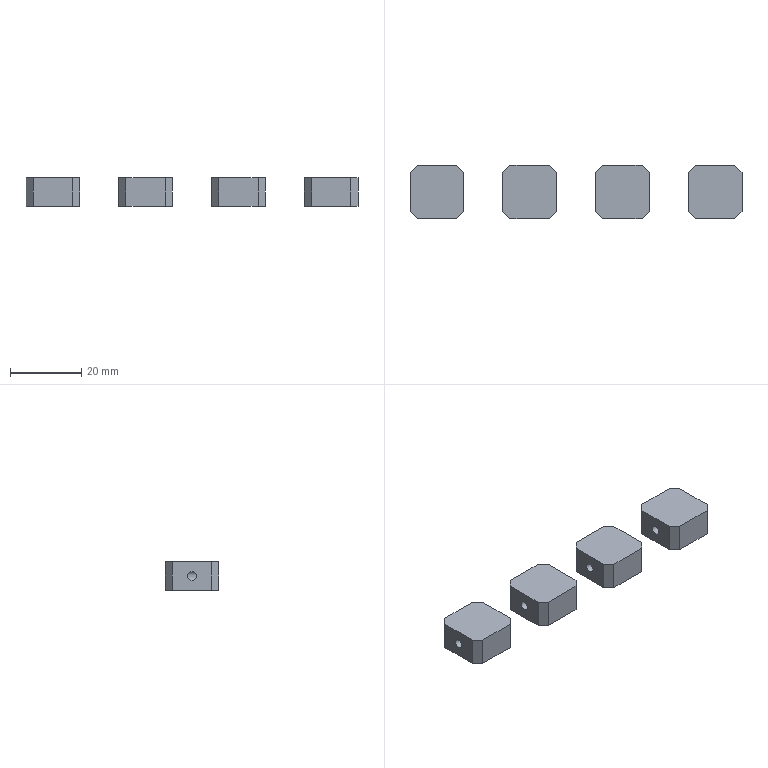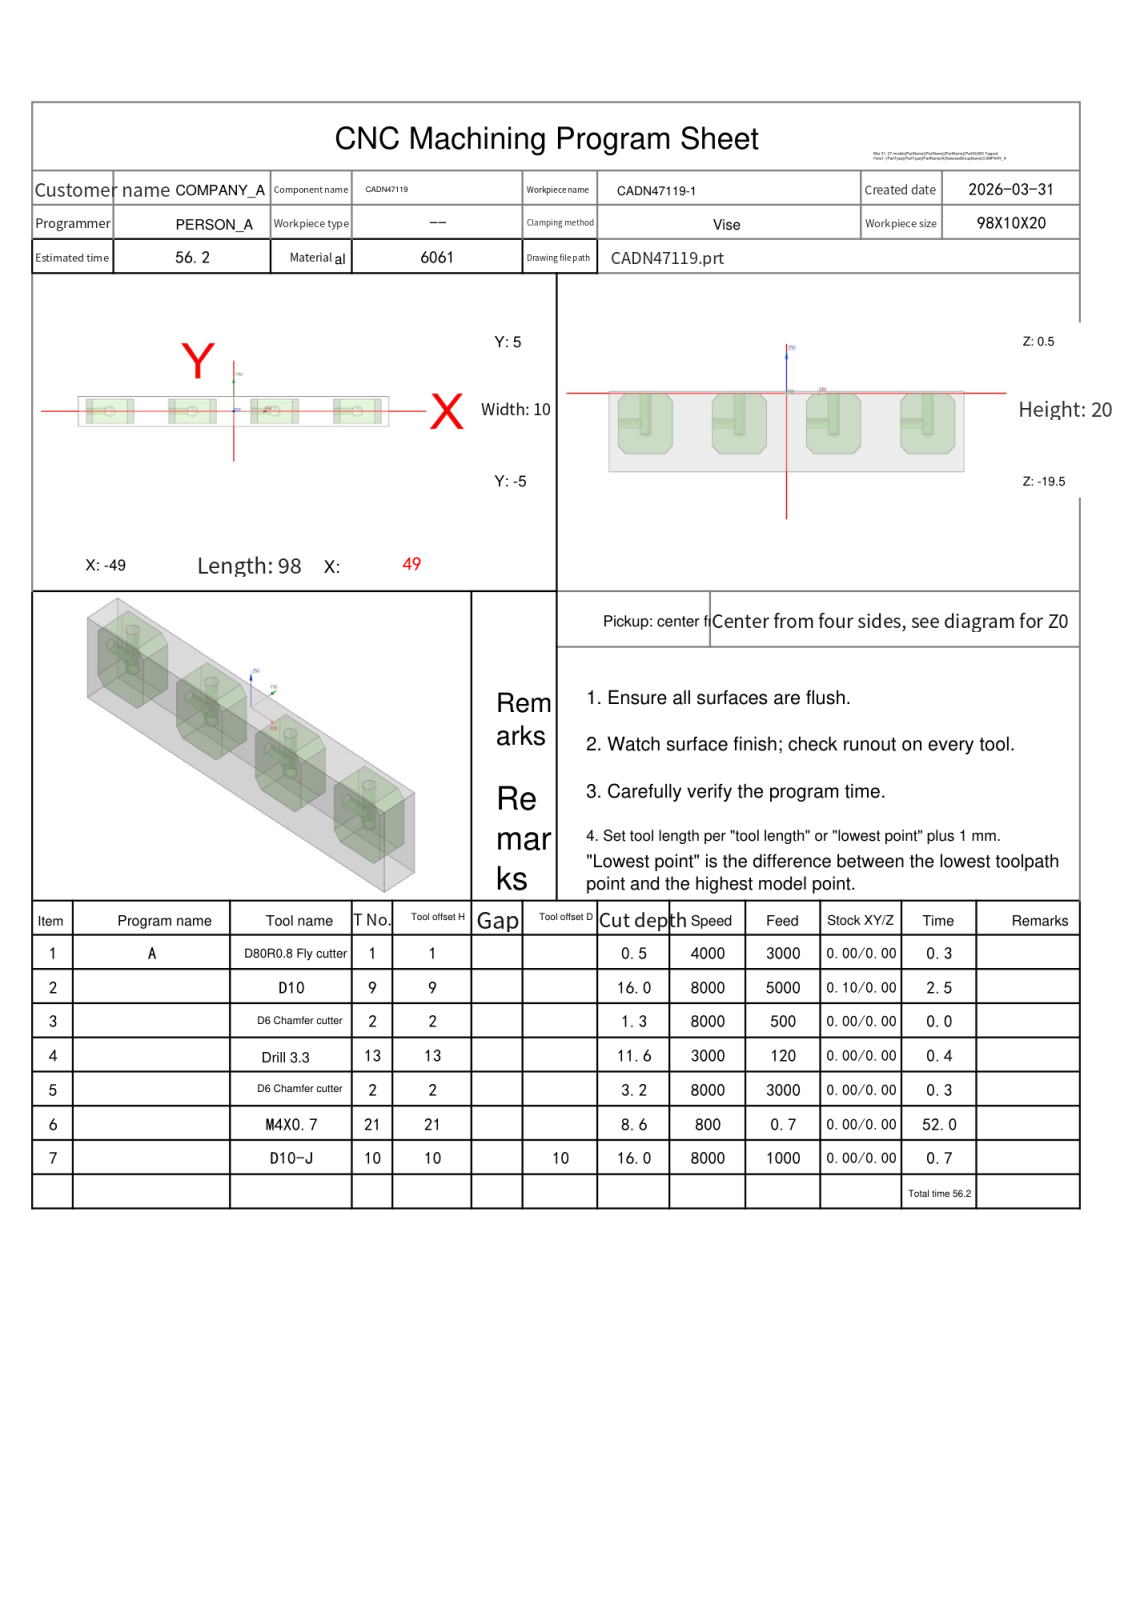NC program | NX | posted by the shop | part box 93 x 15 x 8 mm
Whole program, first 1516 of 2116 lines:
%
O0001
(Machine time: 103.83 MIN)
(===Total Tool:6===)
(T1=D80R0.8 Fly cutter D=80.  R=0.8  D-  H01 Z=-0.   )
(T9=D10     D=10.  R=0.   D-  H09 Z=-15.5 )
(T2=D6 Chamfer cutter   D=6.   R=0.   D-  H02 Z=-2.7  )
(T13=Drill 3.3  D=3.3  DR_a=118 D-  H13 Z=-11.09)
(T21=M4X0.7 D=3.3  DR_a=180 D-  H21 Z=-8.1  )
(T10=D10-J  D=10.  R=0.   D10 H10 Z=-15.5 )
G80 G90 G17 G49 G40
G91 G28 Z0
M01
N1 T01 M06
(D80R0.8 Fly cutter  D=80. R=0.8 H=01 ce=0.20 di=0.10)
G00 G90 G54 X91.5 Y0.0 M03 S4000
G43 H01 Z20.
M08
Z2.1
G01 Z.1 F3000.
X86.5
X-86.5
X-91.5
Z2.1
G00 Z20.
G00 G90 X91.5 Y0.0 M03 S4000
Z20.
Z2.
G01 Z0.0 F1000.
X86.5
X-86.5
X-91.5
Z2.
G00 Z20.
G91 G28 Z0.0
M05
M09
G91 G28 Z0.0
M01
N2 T09 M06
(D10  D=10. R=0. H=09 ce=0.10 di=0.00)
G00 G90 G54 X13. Y9.1 M03 S8000
G43 H09 Z20.
M08
Z.5
G01 X20.5 Z.452 F5000.
G02 X25.6 Y4. Z.401 I0.0 J-5.1
G01 Y-4. Z.349
G02 X20.5 Y-9.1 Z.298 I-5.1 J0.0
G01 X5.5 Z.202
G02 X.4 Y-4. Z.151 I0.0 J5.1
G01 Y4. Z.099
G02 X5.5 Y9.1 Z.048 I5.1 J0.0
G01 X20.5 Z-.048
G02 X25.6 Y4. Z-.099 I0.0 J-5.1
G01 Y-4. Z-.151
G02 X20.5 Y-9.1 Z-.202 I-5.1 J0.0
G01 X5.5 Z-.298
G02 X.4 Y-4. Z-.349 I0.0 J5.1
G01 Y4. Z-.401
G02 X5.5 Y9.1 Z-.452 I5.1 J0.0
G01 X20.5 Z-.548
G02 X25.6 Y4. Z-.599 I0.0 J-5.1
G01 Y-4. Z-.651
G02 X20.5 Y-9.1 Z-.702 I-5.1 J0.0
G01 X5.5 Z-.798
G02 X.4 Y-4. Z-.849 I0.0 J5.1
G01 Y4. Z-.901
G02 X5.5 Y9.1 Z-.952 I5.1 J0.0
G01 X20.5 Z-1.048
G02 X25.6 Y4. Z-1.099 I0.0 J-5.1
G01 Y-4. Z-1.151
G02 X20.5 Y-9.1 Z-1.202 I-5.1 J0.0
G01 X5.5 Z-1.298
G02 X.4 Y-4. Z-1.349 I0.0 J5.1
G01 Y4. Z-1.401
G02 X5.5 Y9.1 Z-1.452 I5.1 J0.0
G01 X20.5 Z-1.548
G02 X25.6 Y4. Z-1.599 I0.0 J-5.1
G01 Y-4. Z-1.651
G02 X20.5 Y-9.1 Z-1.702 I-5.1 J0.0
G01 X5.5 Z-1.798
G02 X.4 Y-4. Z-1.849 I0.0 J5.1
G01 Y4. Z-1.901
G02 X5.5 Y9.1 Z-1.952 I5.1 J0.0
G01 X20.5 Z-2.048
G02 X25.6 Y4. Z-2.099 I0.0 J-5.1
G01 Y-4. Z-2.151
G02 X20.5 Y-9.1 Z-2.202 I-5.1 J0.0
G01 X5.5 Z-2.298
G02 X.4 Y-4. Z-2.349 I0.0 J5.1
G01 Y4. Z-2.401
G02 X5.5 Y9.1 Z-2.452 I5.1 J0.0
G01 X20.5 Z-2.548
G02 X25.6 Y4. Z-2.599 I0.0 J-5.1
G01 Y-4. Z-2.651
G02 X20.5 Y-9.1 Z-2.702 I-5.1 J0.0
G01 X5.5 Z-2.798
G02 X.4 Y-4. Z-2.849 I0.0 J5.1
G01 Y4. Z-2.901
G02 X5.5 Y9.1 Z-2.952 I5.1 J0.0
G01 X20.5 Z-3.048
G02 X25.6 Y4. Z-3.099 I0.0 J-5.1
G01 Y-4. Z-3.151
G02 X20.5 Y-9.1 Z-3.202 I-5.1 J0.0
G01 X5.5 Z-3.298
G02 X.4 Y-4. Z-3.349 I0.0 J5.1
G01 Y4. Z-3.401
G02 X5.5 Y9.1 Z-3.452 I5.1 J0.0
G01 X20.5 Z-3.548
G02 X25.6 Y4. Z-3.599 I0.0 J-5.1
G01 Y-4. Z-3.651
G02 X20.5 Y-9.1 Z-3.702 I-5.1 J0.0
G01 X5.5 Z-3.798
G02 X.4 Y-4. Z-3.849 I0.0 J5.1
G01 Y4. Z-3.901
G02 X5.5 Y9.1 Z-3.952 I5.1 J0.0
G01 X20.5 Z-4.048
G02 X25.6 Y4. Z-4.099 I0.0 J-5.1
G01 Y-4. Z-4.151
G02 X20.5 Y-9.1 Z-4.202 I-5.1 J0.0
G01 X5.5 Z-4.298
G02 X.4 Y-4. Z-4.349 I0.0 J5.1
G01 Y4. Z-4.401
G02 X5.5 Y9.1 Z-4.452 I5.1 J0.0
G01 X20.5 Z-4.548
G02 X25.6 Y4. Z-4.599 I0.0 J-5.1
G01 Y-4. Z-4.651
G02 X20.5 Y-9.1 Z-4.702 I-5.1 J0.0
G01 X5.5 Z-4.798
G02 X.4 Y-4. Z-4.849 I0.0 J5.1
G01 Y4. Z-4.901
G02 X5.5 Y9.1 Z-4.952 I5.1 J0.0
G01 X20.5 Z-5.048
G02 X25.6 Y4. Z-5.099 I0.0 J-5.1
G01 Y-4. Z-5.151
G02 X20.5 Y-9.1 Z-5.202 I-5.1 J0.0
G01 X5.5 Z-5.298
G02 X.4 Y-4. Z-5.349 I0.0 J5.1
G01 Y4. Z-5.401
G02 X5.5 Y9.1 Z-5.452 I5.1 J0.0
G01 X20.5 Z-5.548
G02 X25.6 Y4. Z-5.599 I0.0 J-5.1
G01 Y-4. Z-5.651
G02 X20.5 Y-9.1 Z-5.702 I-5.1 J0.0
G01 X5.5 Z-5.798
G02 X.4 Y-4. Z-5.849 I0.0 J5.1
G01 Y4. Z-5.901
G02 X5.5 Y9.1 Z-5.952 I5.1 J0.0
G01 X20.5 Z-6.048
G02 X25.6 Y4. Z-6.099 I0.0 J-5.1
G01 Y-4. Z-6.151
G02 X20.5 Y-9.1 Z-6.202 I-5.1 J0.0
G01 X5.5 Z-6.298
G02 X.4 Y-4. Z-6.349 I0.0 J5.1
G01 Y4. Z-6.401
G02 X5.5 Y9.1 Z-6.452 I5.1 J0.0
G01 X20.5 Z-6.548
G02 X25.6 Y4. Z-6.599 I0.0 J-5.1
G01 Y-4. Z-6.651
G02 X20.5 Y-9.1 Z-6.702 I-5.1 J0.0
G01 X5.5 Z-6.798
G02 X.4 Y-4. Z-6.849 I0.0 J5.1
G01 Y4. Z-6.901
G02 X5.5 Y9.1 Z-6.952 I5.1 J0.0
G01 X20.5 Z-7.048
G02 X25.6 Y4. Z-7.099 I0.0 J-5.1
G01 Y-4. Z-7.151
G02 X20.5 Y-9.1 Z-7.202 I-5.1 J0.0
G01 X5.5 Z-7.298
G02 X.4 Y-4. Z-7.349 I0.0 J5.1
G01 Y4. Z-7.401
G02 X5.5 Y9.1 Z-7.452 I5.1 J0.0
G01 X20.5 Z-7.548
G02 X25.6 Y4. Z-7.599 I0.0 J-5.1
G01 Y-4. Z-7.651
G02 X20.5 Y-9.1 Z-7.702 I-5.1 J0.0
G01 X5.5 Z-7.798
G02 X.4 Y-4. Z-7.849 I0.0 J5.1
G01 Y4. Z-7.901
G02 X5.5 Y9.1 Z-7.952 I5.1 J0.0
G01 X20.5 Z-8.048
G02 X25.6 Y4. Z-8.099 I0.0 J-5.1
G01 Y-4. Z-8.151
G02 X20.5 Y-9.1 Z-8.202 I-5.1 J0.0
G01 X5.5 Z-8.298
G02 X.4 Y-4. Z-8.349 I0.0 J5.1
G01 Y4. Z-8.401
G02 X5.5 Y9.1 Z-8.452 I5.1 J0.0
G01 X20.5 Z-8.548
G02 X25.6 Y4. Z-8.599 I0.0 J-5.1
G01 Y-4. Z-8.651
G02 X20.5 Y-9.1 Z-8.702 I-5.1 J0.0
G01 X5.5 Z-8.798
G02 X.4 Y-4. Z-8.849 I0.0 J5.1
G01 Y4. Z-8.901
G02 X5.5 Y9.1 Z-8.952 I5.1 J0.0
G01 X20.5 Z-9.048
G02 X25.6 Y4. Z-9.099 I0.0 J-5.1
G01 Y-4. Z-9.151
G02 X20.5 Y-9.1 Z-9.202 I-5.1 J0.0
G01 X5.5 Z-9.298
G02 X.4 Y-4. Z-9.349 I0.0 J5.1
G01 Y4. Z-9.401
G02 X5.5 Y9.1 Z-9.452 I5.1 J0.0
G01 X20.5 Z-9.548
G02 X25.6 Y4. Z-9.599 I0.0 J-5.1
G01 Y-4. Z-9.651
G02 X20.5 Y-9.1 Z-9.702 I-5.1 J0.0
G01 X5.5 Z-9.798
G02 X.4 Y-4. Z-9.849 I0.0 J5.1
G01 Y4. Z-9.901
G02 X5.5 Y9.1 Z-9.952 I5.1 J0.0
G01 X20.5 Z-10.048
G02 X25.6 Y4. Z-10.099 I0.0 J-5.1
G01 Y-4. Z-10.151
G02 X20.5 Y-9.1 Z-10.202 I-5.1 J0.0
G01 X5.5 Z-10.298
G02 X.4 Y-4. Z-10.349 I0.0 J5.1
G01 Y4. Z-10.401
G02 X5.5 Y9.1 Z-10.452 I5.1 J0.0
G01 X20.5 Z-10.548
G02 X25.6 Y4. Z-10.599 I0.0 J-5.1
G01 Y-4. Z-10.651
G02 X20.5 Y-9.1 Z-10.702 I-5.1 J0.0
G01 X5.5 Z-10.798
G02 X.4 Y-4. Z-10.849 I0.0 J5.1
G01 Y4. Z-10.901
G02 X5.5 Y9.1 Z-10.952 I5.1 J0.0
G01 X20.5 Z-11.048
G02 X25.6 Y4. Z-11.099 I0.0 J-5.1
G01 Y-4. Z-11.151
G02 X20.5 Y-9.1 Z-11.202 I-5.1 J0.0
G01 X5.5 Z-11.298
G02 X.4 Y-4. Z-11.349 I0.0 J5.1
G01 Y4. Z-11.401
G02 X5.5 Y9.1 Z-11.452 I5.1 J0.0
G01 X20.5 Z-11.548
G02 X25.6 Y4. Z-11.599 I0.0 J-5.1
G01 Y-4. Z-11.651
G02 X20.5 Y-9.1 Z-11.702 I-5.1 J0.0
G01 X5.5 Z-11.798
G02 X.4 Y-4. Z-11.849 I0.0 J5.1
G01 Y4. Z-11.901
G02 X5.5 Y9.1 Z-11.952 I5.1 J0.0
G01 X20.5 Z-12.048
G02 X25.6 Y4. Z-12.099 I0.0 J-5.1
G01 Y-4. Z-12.151
G02 X20.5 Y-9.1 Z-12.202 I-5.1 J0.0
G01 X5.5 Z-12.298
G02 X.4 Y-4. Z-12.349 I0.0 J5.1
G01 Y4. Z-12.401
G02 X5.5 Y9.1 Z-12.452 I5.1 J0.0
G01 X20.5 Z-12.548
G02 X25.6 Y4. Z-12.599 I0.0 J-5.1
G01 Y-4. Z-12.651
G02 X20.5 Y-9.1 Z-12.702 I-5.1 J0.0
G01 X5.5 Z-12.798
G02 X.4 Y-4. Z-12.849 I0.0 J5.1
G01 Y4. Z-12.901
G02 X5.5 Y9.1 Z-12.952 I5.1 J0.0
G01 X20.5 Z-13.048
G02 X25.6 Y4. Z-13.099 I0.0 J-5.1
G01 Y-4. Z-13.151
G02 X20.5 Y-9.1 Z-13.202 I-5.1 J0.0
G01 X5.5 Z-13.298
G02 X.4 Y-4. Z-13.349 I0.0 J5.1
G01 Y4. Z-13.401
G02 X5.5 Y9.1 Z-13.452 I5.1 J0.0
G01 X20.5 Z-13.548
G02 X25.6 Y4. Z-13.599 I0.0 J-5.1
G01 Y-4. Z-13.651
G02 X20.5 Y-9.1 Z-13.702 I-5.1 J0.0
G01 X5.5 Z-13.798
G02 X.4 Y-4. Z-13.849 I0.0 J5.1
G01 Y4. Z-13.901
G02 X5.5 Y9.1 Z-13.952 I5.1 J0.0
G01 X20.5 Z-14.048
G02 X25.6 Y4. Z-14.099 I0.0 J-5.1
G01 Y-4. Z-14.151
G02 X20.5 Y-9.1 Z-14.202 I-5.1 J0.0
G01 X5.5 Z-14.298
G02 X.4 Y-4. Z-14.349 I0.0 J5.1
G01 Y4. Z-14.401
G02 X5.5 Y9.1 Z-14.452 I5.1 J0.0
G01 X20.5 Z-14.548
G02 X25.6 Y4. Z-14.599 I0.0 J-5.1
G01 Y-4. Z-14.651
G02 X20.5 Y-9.1 Z-14.702 I-5.1 J0.0
G01 X5.5 Z-14.798
G02 X.4 Y-4. Z-14.849 I0.0 J5.1
G01 Y4. Z-14.901
G02 X5.5 Y9.1 Z-14.952 I5.1 J0.0
G01 X20.5 Z-15.048
G02 X25.6 Y4. Z-15.099 I0.0 J-5.1
G01 Y-4. Z-15.151
G02 X20.5 Y-9.1 Z-15.202 I-5.1 J0.0
G01 X5.5 Z-15.298
G02 X.4 Y-4. Z-15.349 I0.0 J5.1
G01 Y4. Z-15.401
G02 X5.5 Y9.1 Z-15.452 I5.1 J0.0
G01 X13. Z-15.5
X20.5
G02 X25.6 Y4. I0.0 J-5.1
G01 Y-4.
G02 X20.5 Y-9.1 I-5.1 J0.0
G01 X5.5
G02 X.4 Y-4. I0.0 J5.1
G01 Y4.
G02 X5.5 Y9.1 I5.1 J0.0
G01 X13.
X13.5
Z-14.5
G00 Z20.
X39.
Z.5
G01 X46.5 Z.452
G02 X51.6 Y4. Z.401 I0.0 J-5.1
G01 Y-4. Z.349
G02 X46.5 Y-9.1 Z.298 I-5.1 J0.0
G01 X31.5 Z.202
G02 X26.4 Y-4. Z.151 I0.0 J5.1
G01 Y4. Z.099
G02 X31.5 Y9.1 Z.048 I5.1 J0.0
G01 X46.5 Z-.048
G02 X51.6 Y4. Z-.099 I0.0 J-5.1
G01 Y-4. Z-.151
G02 X46.5 Y-9.1 Z-.202 I-5.1 J0.0
G01 X31.5 Z-.298
G02 X26.4 Y-4. Z-.349 I0.0 J5.1
G01 Y4. Z-.401
G02 X31.5 Y9.1 Z-.452 I5.1 J0.0
G01 X46.5 Z-.548
G02 X51.6 Y4. Z-.599 I0.0 J-5.1
G01 Y-4. Z-.651
G02 X46.5 Y-9.1 Z-.702 I-5.1 J0.0
G01 X31.5 Z-.798
G02 X26.4 Y-4. Z-.849 I0.0 J5.1
G01 Y4. Z-.901
G02 X31.5 Y9.1 Z-.952 I5.1 J0.0
G01 X46.5 Z-1.048
G02 X51.6 Y4. Z-1.099 I0.0 J-5.1
G01 Y-4. Z-1.151
G02 X46.5 Y-9.1 Z-1.202 I-5.1 J0.0
G01 X31.5 Z-1.298
G02 X26.4 Y-4. Z-1.349 I0.0 J5.1
G01 Y4. Z-1.401
G02 X31.5 Y9.1 Z-1.452 I5.1 J0.0
G01 X46.5 Z-1.548
G02 X51.6 Y4. Z-1.599 I0.0 J-5.1
G01 Y-4. Z-1.651
G02 X46.5 Y-9.1 Z-1.702 I-5.1 J0.0
G01 X31.5 Z-1.798
G02 X26.4 Y-4. Z-1.849 I0.0 J5.1
G01 Y4. Z-1.901
G02 X31.5 Y9.1 Z-1.952 I5.1 J0.0
G01 X46.5 Z-2.048
G02 X51.6 Y4. Z-2.099 I0.0 J-5.1
G01 Y-4. Z-2.151
G02 X46.5 Y-9.1 Z-2.202 I-5.1 J0.0
G01 X31.5 Z-2.298
G02 X26.4 Y-4. Z-2.349 I0.0 J5.1
G01 Y4. Z-2.401
G02 X31.5 Y9.1 Z-2.452 I5.1 J0.0
G01 X46.5 Z-2.548
G02 X51.6 Y4. Z-2.599 I0.0 J-5.1
G01 Y-4. Z-2.651
G02 X46.5 Y-9.1 Z-2.702 I-5.1 J0.0
G01 X31.5 Z-2.798
G02 X26.4 Y-4. Z-2.849 I0.0 J5.1
G01 Y4. Z-2.901
G02 X31.5 Y9.1 Z-2.952 I5.1 J0.0
G01 X46.5 Z-3.048
G02 X51.6 Y4. Z-3.099 I0.0 J-5.1
G01 Y-4. Z-3.151
G02 X46.5 Y-9.1 Z-3.202 I-5.1 J0.0
G01 X31.5 Z-3.298
G02 X26.4 Y-4. Z-3.349 I0.0 J5.1
G01 Y4. Z-3.401
G02 X31.5 Y9.1 Z-3.452 I5.1 J0.0
G01 X46.5 Z-3.548
G02 X51.6 Y4. Z-3.599 I0.0 J-5.1
G01 Y-4. Z-3.651
G02 X46.5 Y-9.1 Z-3.702 I-5.1 J0.0
G01 X31.5 Z-3.798
G02 X26.4 Y-4. Z-3.849 I0.0 J5.1
G01 Y4. Z-3.901
G02 X31.5 Y9.1 Z-3.952 I5.1 J0.0
G01 X46.5 Z-4.048
G02 X51.6 Y4. Z-4.099 I0.0 J-5.1
G01 Y-4. Z-4.151
G02 X46.5 Y-9.1 Z-4.202 I-5.1 J0.0
G01 X31.5 Z-4.298
G02 X26.4 Y-4. Z-4.349 I0.0 J5.1
G01 Y4. Z-4.401
G02 X31.5 Y9.1 Z-4.452 I5.1 J0.0
G01 X46.5 Z-4.548
G02 X51.6 Y4. Z-4.599 I0.0 J-5.1
G01 Y-4. Z-4.651
G02 X46.5 Y-9.1 Z-4.702 I-5.1 J0.0
G01 X31.5 Z-4.798
G02 X26.4 Y-4. Z-4.849 I0.0 J5.1
G01 Y4. Z-4.901
G02 X31.5 Y9.1 Z-4.952 I5.1 J0.0
G01 X46.5 Z-5.048
G02 X51.6 Y4. Z-5.099 I0.0 J-5.1
G01 Y-4. Z-5.151
G02 X46.5 Y-9.1 Z-5.202 I-5.1 J0.0
G01 X31.5 Z-5.298
G02 X26.4 Y-4. Z-5.349 I0.0 J5.1
G01 Y4. Z-5.401
G02 X31.5 Y9.1 Z-5.452 I5.1 J0.0
G01 X46.5 Z-5.548
G02 X51.6 Y4. Z-5.599 I0.0 J-5.1
G01 Y-4. Z-5.651
G02 X46.5 Y-9.1 Z-5.702 I-5.1 J0.0
G01 X31.5 Z-5.798
G02 X26.4 Y-4. Z-5.849 I0.0 J5.1
G01 Y4. Z-5.901
G02 X31.5 Y9.1 Z-5.952 I5.1 J0.0
G01 X46.5 Z-6.048
G02 X51.6 Y4. Z-6.099 I0.0 J-5.1
G01 Y-4. Z-6.151
G02 X46.5 Y-9.1 Z-6.202 I-5.1 J0.0
G01 X31.5 Z-6.298
G02 X26.4 Y-4. Z-6.349 I0.0 J5.1
G01 Y4. Z-6.401
G02 X31.5 Y9.1 Z-6.452 I5.1 J0.0
G01 X46.5 Z-6.548
G02 X51.6 Y4. Z-6.599 I0.0 J-5.1
G01 Y-4. Z-6.651
G02 X46.5 Y-9.1 Z-6.702 I-5.1 J0.0
G01 X31.5 Z-6.798
G02 X26.4 Y-4. Z-6.849 I0.0 J5.1
G01 Y4. Z-6.901
G02 X31.5 Y9.1 Z-6.952 I5.1 J0.0
G01 X46.5 Z-7.048
G02 X51.6 Y4. Z-7.099 I0.0 J-5.1
G01 Y-4. Z-7.151
G02 X46.5 Y-9.1 Z-7.202 I-5.1 J0.0
G01 X31.5 Z-7.298
G02 X26.4 Y-4. Z-7.349 I0.0 J5.1
G01 Y4. Z-7.401
G02 X31.5 Y9.1 Z-7.452 I5.1 J0.0
G01 X46.5 Z-7.548
G02 X51.6 Y4. Z-7.599 I0.0 J-5.1
G01 Y-4. Z-7.651
G02 X46.5 Y-9.1 Z-7.702 I-5.1 J0.0
G01 X31.5 Z-7.798
G02 X26.4 Y-4. Z-7.849 I0.0 J5.1
G01 Y4. Z-7.901
G02 X31.5 Y9.1 Z-7.952 I5.1 J0.0
G01 X46.5 Z-8.048
G02 X51.6 Y4. Z-8.099 I0.0 J-5.1
G01 Y-4. Z-8.151
G02 X46.5 Y-9.1 Z-8.202 I-5.1 J0.0
G01 X31.5 Z-8.298
G02 X26.4 Y-4. Z-8.349 I0.0 J5.1
G01 Y4. Z-8.401
G02 X31.5 Y9.1 Z-8.452 I5.1 J0.0
G01 X46.5 Z-8.548
G02 X51.6 Y4. Z-8.599 I0.0 J-5.1
G01 Y-4. Z-8.651
G02 X46.5 Y-9.1 Z-8.702 I-5.1 J0.0
G01 X31.5 Z-8.798
G02 X26.4 Y-4. Z-8.849 I0.0 J5.1
G01 Y4. Z-8.901
G02 X31.5 Y9.1 Z-8.952 I5.1 J0.0
G01 X46.5 Z-9.048
G02 X51.6 Y4. Z-9.099 I0.0 J-5.1
G01 Y-4. Z-9.151
G02 X46.5 Y-9.1 Z-9.202 I-5.1 J0.0
G01 X31.5 Z-9.298
G02 X26.4 Y-4. Z-9.349 I0.0 J5.1
G01 Y4. Z-9.401
G02 X31.5 Y9.1 Z-9.452 I5.1 J0.0
G01 X46.5 Z-9.548
G02 X51.6 Y4. Z-9.599 I0.0 J-5.1
G01 Y-4. Z-9.651
G02 X46.5 Y-9.1 Z-9.702 I-5.1 J0.0
G01 X31.5 Z-9.798
G02 X26.4 Y-4. Z-9.849 I0.0 J5.1
G01 Y4. Z-9.901
G02 X31.5 Y9.1 Z-9.952 I5.1 J0.0
G01 X46.5 Z-10.048
G02 X51.6 Y4. Z-10.099 I0.0 J-5.1
G01 Y-4. Z-10.151
G02 X46.5 Y-9.1 Z-10.202 I-5.1 J0.0
G01 X31.5 Z-10.298
G02 X26.4 Y-4. Z-10.349 I0.0 J5.1
G01 Y4. Z-10.401
G02 X31.5 Y9.1 Z-10.452 I5.1 J0.0
G01 X46.5 Z-10.548
G02 X51.6 Y4. Z-10.599 I0.0 J-5.1
G01 Y-4. Z-10.651
G02 X46.5 Y-9.1 Z-10.702 I-5.1 J0.0
G01 X31.5 Z-10.798
G02 X26.4 Y-4. Z-10.849 I0.0 J5.1
G01 Y4. Z-10.901
G02 X31.5 Y9.1 Z-10.952 I5.1 J0.0
G01 X46.5 Z-11.048
G02 X51.6 Y4. Z-11.099 I0.0 J-5.1
G01 Y-4. Z-11.151
G02 X46.5 Y-9.1 Z-11.202 I-5.1 J0.0
G01 X31.5 Z-11.298
G02 X26.4 Y-4. Z-11.349 I0.0 J5.1
G01 Y4. Z-11.401
G02 X31.5 Y9.1 Z-11.452 I5.1 J0.0
G01 X46.5 Z-11.548
G02 X51.6 Y4. Z-11.599 I0.0 J-5.1
G01 Y-4. Z-11.651
G02 X46.5 Y-9.1 Z-11.702 I-5.1 J0.0
G01 X31.5 Z-11.798
G02 X26.4 Y-4. Z-11.849 I0.0 J5.1
G01 Y4. Z-11.901
G02 X31.5 Y9.1 Z-11.952 I5.1 J0.0
G01 X46.5 Z-12.048
G02 X51.6 Y4. Z-12.099 I0.0 J-5.1
G01 Y-4. Z-12.151
G02 X46.5 Y-9.1 Z-12.202 I-5.1 J0.0
G01 X31.5 Z-12.298
G02 X26.4 Y-4. Z-12.349 I0.0 J5.1
G01 Y4. Z-12.401
G02 X31.5 Y9.1 Z-12.452 I5.1 J0.0
G01 X46.5 Z-12.548
G02 X51.6 Y4. Z-12.599 I0.0 J-5.1
G01 Y-4. Z-12.651
G02 X46.5 Y-9.1 Z-12.702 I-5.1 J0.0
G01 X31.5 Z-12.798
G02 X26.4 Y-4. Z-12.849 I0.0 J5.1
G01 Y4. Z-12.901
G02 X31.5 Y9.1 Z-12.952 I5.1 J0.0
G01 X46.5 Z-13.048
G02 X51.6 Y4. Z-13.099 I0.0 J-5.1
G01 Y-4. Z-13.151
G02 X46.5 Y-9.1 Z-13.202 I-5.1 J0.0
G01 X31.5 Z-13.298
G02 X26.4 Y-4. Z-13.349 I0.0 J5.1
G01 Y4. Z-13.401
G02 X31.5 Y9.1 Z-13.452 I5.1 J0.0
G01 X46.5 Z-13.548
G02 X51.6 Y4. Z-13.599 I0.0 J-5.1
G01 Y-4. Z-13.651
G02 X46.5 Y-9.1 Z-13.702 I-5.1 J0.0
G01 X31.5 Z-13.798
G02 X26.4 Y-4. Z-13.849 I0.0 J5.1
G01 Y4. Z-13.901
G02 X31.5 Y9.1 Z-13.952 I5.1 J0.0
G01 X46.5 Z-14.048
G02 X51.6 Y4. Z-14.099 I0.0 J-5.1
G01 Y-4. Z-14.151
G02 X46.5 Y-9.1 Z-14.202 I-5.1 J0.0
G01 X31.5 Z-14.298
G02 X26.4 Y-4. Z-14.349 I0.0 J5.1
G01 Y4. Z-14.401
G02 X31.5 Y9.1 Z-14.452 I5.1 J0.0
G01 X46.5 Z-14.548
G02 X51.6 Y4. Z-14.599 I0.0 J-5.1
G01 Y-4. Z-14.651
G02 X46.5 Y-9.1 Z-14.702 I-5.1 J0.0
G01 X31.5 Z-14.798
G02 X26.4 Y-4. Z-14.849 I0.0 J5.1
G01 Y4. Z-14.901
G02 X31.5 Y9.1 Z-14.952 I5.1 J0.0
G01 X46.5 Z-15.048
G02 X51.6 Y4. Z-15.099 I0.0 J-5.1
G01 Y-4. Z-15.151
G02 X46.5 Y-9.1 Z-15.202 I-5.1 J0.0
G01 X31.5 Z-15.298
G02 X26.4 Y-4. Z-15.349 I0.0 J5.1
G01 Y4. Z-15.401
G02 X31.5 Y9.1 Z-15.452 I5.1 J0.0
G01 X39. Z-15.5
X46.5
G02 X51.6 Y4. I0.0 J-5.1
G01 Y-4.
G02 X46.5 Y-9.1 I-5.1 J0.0
G01 X31.5
G02 X26.4 Y-4. I0.0 J5.1
G01 Y4.
G02 X31.5 Y9.1 I5.1 J0.0
G01 X39.
X39.5
Z-14.5
G00 Z20.
X-13.
Z.5
G01 X-5.5 Z.452
G02 X-.4 Y4. Z.401 I0.0 J-5.1
G01 Y-4. Z.349
G02 X-5.5 Y-9.1 Z.298 I-5.1 J0.0
G01 X-20.5 Z.202
G02 X-25.6 Y-4. Z.151 I0.0 J5.1
G01 Y4. Z.099
G02 X-20.5 Y9.1 Z.048 I5.1 J0.0
G01 X-5.5 Z-.048
G02 X-.4 Y4. Z-.099 I0.0 J-5.1
G01 Y-4. Z-.151
G02 X-5.5 Y-9.1 Z-.202 I-5.1 J0.0
G01 X-20.5 Z-.298
G02 X-25.6 Y-4. Z-.349 I0.0 J5.1
G01 Y4. Z-.401
G02 X-20.5 Y9.1 Z-.452 I5.1 J0.0
G01 X-5.5 Z-.548
G02 X-.4 Y4. Z-.599 I0.0 J-5.1
G01 Y-4. Z-.651
G02 X-5.5 Y-9.1 Z-.702 I-5.1 J0.0
G01 X-20.5 Z-.798
G02 X-25.6 Y-4. Z-.849 I0.0 J5.1
G01 Y4. Z-.901
G02 X-20.5 Y9.1 Z-.952 I5.1 J0.0
G01 X-5.5 Z-1.048
G02 X-.4 Y4. Z-1.099 I0.0 J-5.1
G01 Y-4. Z-1.151
G02 X-5.5 Y-9.1 Z-1.202 I-5.1 J0.0
G01 X-20.5 Z-1.298
G02 X-25.6 Y-4. Z-1.349 I0.0 J5.1
G01 Y4. Z-1.401
G02 X-20.5 Y9.1 Z-1.452 I5.1 J0.0
G01 X-5.5 Z-1.548
G02 X-.4 Y4. Z-1.599 I0.0 J-5.1
G01 Y-4. Z-1.651
G02 X-5.5 Y-9.1 Z-1.702 I-5.1 J0.0
G01 X-20.5 Z-1.798
G02 X-25.6 Y-4. Z-1.849 I0.0 J5.1
G01 Y4. Z-1.901
G02 X-20.5 Y9.1 Z-1.952 I5.1 J0.0
G01 X-5.5 Z-2.048
G02 X-.4 Y4. Z-2.099 I0.0 J-5.1
G01 Y-4. Z-2.151
G02 X-5.5 Y-9.1 Z-2.202 I-5.1 J0.0
G01 X-20.5 Z-2.298
G02 X-25.6 Y-4. Z-2.349 I0.0 J5.1
G01 Y4. Z-2.401
G02 X-20.5 Y9.1 Z-2.452 I5.1 J0.0
G01 X-5.5 Z-2.548
G02 X-.4 Y4. Z-2.599 I0.0 J-5.1
G01 Y-4. Z-2.651
G02 X-5.5 Y-9.1 Z-2.702 I-5.1 J0.0
G01 X-20.5 Z-2.798
G02 X-25.6 Y-4. Z-2.849 I0.0 J5.1
G01 Y4. Z-2.901
G02 X-20.5 Y9.1 Z-2.952 I5.1 J0.0
G01 X-5.5 Z-3.048
G02 X-.4 Y4. Z-3.099 I0.0 J-5.1
G01 Y-4. Z-3.151
G02 X-5.5 Y-9.1 Z-3.202 I-5.1 J0.0
G01 X-20.5 Z-3.298
G02 X-25.6 Y-4. Z-3.349 I0.0 J5.1
G01 Y4. Z-3.401
G02 X-20.5 Y9.1 Z-3.452 I5.1 J0.0
G01 X-5.5 Z-3.548
G02 X-.4 Y4. Z-3.599 I0.0 J-5.1
G01 Y-4. Z-3.651
G02 X-5.5 Y-9.1 Z-3.702 I-5.1 J0.0
G01 X-20.5 Z-3.798
G02 X-25.6 Y-4. Z-3.849 I0.0 J5.1
G01 Y4. Z-3.901
G02 X-20.5 Y9.1 Z-3.952 I5.1 J0.0
G01 X-5.5 Z-4.048
G02 X-.4 Y4. Z-4.099 I0.0 J-5.1
G01 Y-4. Z-4.151
G02 X-5.5 Y-9.1 Z-4.202 I-5.1 J0.0
G01 X-20.5 Z-4.298
G02 X-25.6 Y-4. Z-4.349 I0.0 J5.1
G01 Y4. Z-4.401
G02 X-20.5 Y9.1 Z-4.452 I5.1 J0.0
G01 X-5.5 Z-4.548
G02 X-.4 Y4. Z-4.599 I0.0 J-5.1
G01 Y-4. Z-4.651
G02 X-5.5 Y-9.1 Z-4.702 I-5.1 J0.0
G01 X-20.5 Z-4.798
G02 X-25.6 Y-4. Z-4.849 I0.0 J5.1
G01 Y4. Z-4.901
G02 X-20.5 Y9.1 Z-4.952 I5.1 J0.0
G01 X-5.5 Z-5.048
G02 X-.4 Y4. Z-5.099 I0.0 J-5.1
G01 Y-4. Z-5.151
G02 X-5.5 Y-9.1 Z-5.202 I-5.1 J0.0
G01 X-20.5 Z-5.298
G02 X-25.6 Y-4. Z-5.349 I0.0 J5.1
G01 Y4. Z-5.401
G02 X-20.5 Y9.1 Z-5.452 I5.1 J0.0
G01 X-5.5 Z-5.548
G02 X-.4 Y4. Z-5.599 I0.0 J-5.1
G01 Y-4. Z-5.651
G02 X-5.5 Y-9.1 Z-5.702 I-5.1 J0.0
G01 X-20.5 Z-5.798
G02 X-25.6 Y-4. Z-5.849 I0.0 J5.1
G01 Y4. Z-5.901
G02 X-20.5 Y9.1 Z-5.952 I5.1 J0.0
G01 X-5.5 Z-6.048
G02 X-.4 Y4. Z-6.099 I0.0 J-5.1
G01 Y-4. Z-6.151
G02 X-5.5 Y-9.1 Z-6.202 I-5.1 J0.0
G01 X-20.5 Z-6.298
G02 X-25.6 Y-4. Z-6.349 I0.0 J5.1
G01 Y4. Z-6.401
G02 X-20.5 Y9.1 Z-6.452 I5.1 J0.0
G01 X-5.5 Z-6.548
G02 X-.4 Y4. Z-6.599 I0.0 J-5.1
G01 Y-4. Z-6.651
G02 X-5.5 Y-9.1 Z-6.702 I-5.1 J0.0
G01 X-20.5 Z-6.798
G02 X-25.6 Y-4. Z-6.849 I0.0 J5.1
G01 Y4. Z-6.901
G02 X-20.5 Y9.1 Z-6.952 I5.1 J0.0
G01 X-5.5 Z-7.048
G02 X-.4 Y4. Z-7.099 I0.0 J-5.1
G01 Y-4. Z-7.151
G02 X-5.5 Y-9.1 Z-7.202 I-5.1 J0.0
G01 X-20.5 Z-7.298
G02 X-25.6 Y-4. Z-7.349 I0.0 J5.1
G01 Y4. Z-7.401
G02 X-20.5 Y9.1 Z-7.452 I5.1 J0.0
G01 X-5.5 Z-7.548
G02 X-.4 Y4. Z-7.599 I0.0 J-5.1
G01 Y-4. Z-7.651
G02 X-5.5 Y-9.1 Z-7.702 I-5.1 J0.0
G01 X-20.5 Z-7.798
G02 X-25.6 Y-4. Z-7.849 I0.0 J5.1
G01 Y4. Z-7.901
G02 X-20.5 Y9.1 Z-7.952 I5.1 J0.0
G01 X-5.5 Z-8.048
G02 X-.4 Y4. Z-8.099 I0.0 J-5.1
G01 Y-4. Z-8.151
G02 X-5.5 Y-9.1 Z-8.202 I-5.1 J0.0
G01 X-20.5 Z-8.298
G02 X-25.6 Y-4. Z-8.349 I0.0 J5.1
G01 Y4. Z-8.401
G02 X-20.5 Y9.1 Z-8.452 I5.1 J0.0
G01 X-5.5 Z-8.548
G02 X-.4 Y4. Z-8.599 I0.0 J-5.1
G01 Y-4. Z-8.651
G02 X-5.5 Y-9.1 Z-8.702 I-5.1 J0.0
G01 X-20.5 Z-8.798
G02 X-25.6 Y-4. Z-8.849 I0.0 J5.1
G01 Y4. Z-8.901
G02 X-20.5 Y9.1 Z-8.952 I5.1 J0.0
G01 X-5.5 Z-9.048
G02 X-.4 Y4. Z-9.099 I0.0 J-5.1
G01 Y-4. Z-9.151
G02 X-5.5 Y-9.1 Z-9.202 I-5.1 J0.0
G01 X-20.5 Z-9.298
G02 X-25.6 Y-4. Z-9.349 I0.0 J5.1
G01 Y4. Z-9.401
G02 X-20.5 Y9.1 Z-9.452 I5.1 J0.0
G01 X-5.5 Z-9.548
G02 X-.4 Y4. Z-9.599 I0.0 J-5.1
G01 Y-4. Z-9.651
G02 X-5.5 Y-9.1 Z-9.702 I-5.1 J0.0
G01 X-20.5 Z-9.798
G02 X-25.6 Y-4. Z-9.849 I0.0 J5.1
G01 Y4. Z-9.901
G02 X-20.5 Y9.1 Z-9.952 I5.1 J0.0
G01 X-5.5 Z-10.048
G02 X-.4 Y4. Z-10.099 I0.0 J-5.1
G01 Y-4. Z-10.151
G02 X-5.5 Y-9.1 Z-10.202 I-5.1 J0.0
G01 X-20.5 Z-10.298
G02 X-25.6 Y-4. Z-10.349 I0.0 J5.1
G01 Y4. Z-10.401
G02 X-20.5 Y9.1 Z-10.452 I5.1 J0.0
G01 X-5.5 Z-10.548
G02 X-.4 Y4. Z-10.599 I0.0 J-5.1
G01 Y-4. Z-10.651
G02 X-5.5 Y-9.1 Z-10.702 I-5.1 J0.0
G01 X-20.5 Z-10.798
G02 X-25.6 Y-4. Z-10.849 I0.0 J5.1
G01 Y4. Z-10.901
G02 X-20.5 Y9.1 Z-10.952 I5.1 J0.0
G01 X-5.5 Z-11.048
G02 X-.4 Y4. Z-11.099 I0.0 J-5.1
G01 Y-4. Z-11.151
G02 X-5.5 Y-9.1 Z-11.202 I-5.1 J0.0
G01 X-20.5 Z-11.298
G02 X-25.6 Y-4. Z-11.349 I0.0 J5.1
G01 Y4. Z-11.401
G02 X-20.5 Y9.1 Z-11.452 I5.1 J0.0
G01 X-5.5 Z-11.548
G02 X-.4 Y4. Z-11.599 I0.0 J-5.1
G01 Y-4. Z-11.651
G02 X-5.5 Y-9.1 Z-11.702 I-5.1 J0.0
G01 X-20.5 Z-11.798
G02 X-25.6 Y-4. Z-11.849 I0.0 J5.1
G01 Y4. Z-11.901
G02 X-20.5 Y9.1 Z-11.952 I5.1 J0.0
G01 X-5.5 Z-12.048
G02 X-.4 Y4. Z-12.099 I0.0 J-5.1
G01 Y-4. Z-12.151
G02 X-5.5 Y-9.1 Z-12.202 I-5.1 J0.0
G01 X-20.5 Z-12.298
G02 X-25.6 Y-4. Z-12.349 I0.0 J5.1
G01 Y4. Z-12.401
G02 X-20.5 Y9.1 Z-12.452 I5.1 J0.0
G01 X-5.5 Z-12.548
G02 X-.4 Y4. Z-12.599 I0.0 J-5.1
G01 Y-4. Z-12.651
G02 X-5.5 Y-9.1 Z-12.702 I-5.1 J0.0
G01 X-20.5 Z-12.798
G02 X-25.6 Y-4. Z-12.849 I0.0 J5.1
G01 Y4. Z-12.901
G02 X-20.5 Y9.1 Z-12.952 I5.1 J0.0
G01 X-5.5 Z-13.048
G02 X-.4 Y4. Z-13.099 I0.0 J-5.1
G01 Y-4. Z-13.151
G02 X-5.5 Y-9.1 Z-13.202 I-5.1 J0.0
G01 X-20.5 Z-13.298
G02 X-25.6 Y-4. Z-13.349 I0.0 J5.1
G01 Y4. Z-13.401
G02 X-20.5 Y9.1 Z-13.452 I5.1 J0.0
G01 X-5.5 Z-13.548
G02 X-.4 Y4. Z-13.599 I0.0 J-5.1
G01 Y-4. Z-13.651
G02 X-5.5 Y-9.1 Z-13.702 I-5.1 J0.0
G01 X-20.5 Z-13.798
G02 X-25.6 Y-4. Z-13.849 I0.0 J5.1
G01 Y4. Z-13.901
G02 X-20.5 Y9.1 Z-13.952 I5.1 J0.0
G01 X-5.5 Z-14.048
G02 X-.4 Y4. Z-14.099 I0.0 J-5.1
G01 Y-4. Z-14.151
G02 X-5.5 Y-9.1 Z-14.202 I-5.1 J0.0
G01 X-20.5 Z-14.298
G02 X-25.6 Y-4. Z-14.349 I0.0 J5.1
G01 Y4. Z-14.401
G02 X-20.5 Y9.1 Z-14.452 I5.1 J0.0
G01 X-5.5 Z-14.548
G02 X-.4 Y4. Z-14.599 I0.0 J-5.1
G01 Y-4. Z-14.651
G02 X-5.5 Y-9.1 Z-14.702 I-5.1 J0.0
G01 X-20.5 Z-14.798
G02 X-25.6 Y-4. Z-14.849 I0.0 J5.1
G01 Y4. Z-14.901
G02 X-20.5 Y9.1 Z-14.952 I5.1 J0.0
G01 X-5.5 Z-15.048
G02 X-.4 Y4. Z-15.099 I0.0 J-5.1
G01 Y-4. Z-15.151
G02 X-5.5 Y-9.1 Z-15.202 I-5.1 J0.0
G01 X-20.5 Z-15.298
G02 X-25.6 Y-4. Z-15.349 I0.0 J5.1
G01 Y4. Z-15.401
G02 X-20.5 Y9.1 Z-15.452 I5.1 J0.0
G01 X-13. Z-15.5
X-5.5
G02 X-.4 Y4. I0.0 J-5.1
G01 Y-4.
G02 X-5.5 Y-9.1 I-5.1 J0.0
G01 X-20.5
G02 X-25.6 Y-4. I0.0 J5.1
G01 Y4.
G02 X-20.5 Y9.1 I5.1 J0.0
G01 X-13.
X-12.5
Z-14.5
G00 Z20.
X-39.
Z.5
G01 X-31.5 Z.452
G02 X-26.4 Y4. Z.401 I0.0 J-5.1
G01 Y-4. Z.349
G02 X-31.5 Y-9.1 Z.298 I-5.1 J0.0
G01 X-46.5 Z.202
G02 X-51.6 Y-4. Z.151 I0.0 J5.1
G01 Y4. Z.099
G02 X-46.5 Y9.1 Z.048 I5.1 J0.0
G01 X-31.5 Z-.048
G02 X-26.4 Y4. Z-.099 I0.0 J-5.1
G01 Y-4. Z-.151
G02 X-31.5 Y-9.1 Z-.202 I-5.1 J0.0
G01 X-46.5 Z-.298
G02 X-51.6 Y-4. Z-.349 I0.0 J5.1
G01 Y4. Z-.401
G02 X-46.5 Y9.1 Z-.452 I5.1 J0.0
G01 X-31.5 Z-.548
G02 X-26.4 Y4. Z-.599 I0.0 J-5.1
G01 Y-4. Z-.651
G02 X-31.5 Y-9.1 Z-.702 I-5.1 J0.0
G01 X-46.5 Z-.798
G02 X-51.6 Y-4. Z-.849 I0.0 J5.1
G01 Y4. Z-.901
G02 X-46.5 Y9.1 Z-.952 I5.1 J0.0
G01 X-31.5 Z-1.048
G02 X-26.4 Y4. Z-1.099 I0.0 J-5.1
G01 Y-4. Z-1.151
G02 X-31.5 Y-9.1 Z-1.202 I-5.1 J0.0
G01 X-46.5 Z-1.298
G02 X-51.6 Y-4. Z-1.349 I0.0 J5.1
G01 Y4. Z-1.401
G02 X-46.5 Y9.1 Z-1.452 I5.1 J0.0
G01 X-31.5 Z-1.548
G02 X-26.4 Y4. Z-1.599 I0.0 J-5.1
G01 Y-4. Z-1.651
G02 X-31.5 Y-9.1 Z-1.702 I-5.1 J0.0
G01 X-46.5 Z-1.798
G02 X-51.6 Y-4. Z-1.849 I0.0 J5.1
G01 Y4. Z-1.901
G02 X-46.5 Y9.1 Z-1.952 I5.1 J0.0
G01 X-31.5 Z-2.048
G02 X-26.4 Y4. Z-2.099 I0.0 J-5.1
G01 Y-4. Z-2.151
G02 X-31.5 Y-9.1 Z-2.202 I-5.1 J0.0
G01 X-46.5 Z-2.298
G02 X-51.6 Y-4. Z-2.349 I0.0 J5.1
G01 Y4. Z-2.401
G02 X-46.5 Y9.1 Z-2.452 I5.1 J0.0
G01 X-31.5 Z-2.548
G02 X-26.4 Y4. Z-2.599 I0.0 J-5.1
G01 Y-4. Z-2.651
G02 X-31.5 Y-9.1 Z-2.702 I-5.1 J0.0
G01 X-46.5 Z-2.798
G02 X-51.6 Y-4. Z-2.849 I0.0 J5.1
G01 Y4. Z-2.901
G02 X-46.5 Y9.1 Z-2.952 I5.1 J0.0
G01 X-31.5 Z-3.048
G02 X-26.4 Y4. Z-3.099 I0.0 J-5.1
G01 Y-4. Z-3.151
G02 X-31.5 Y-9.1 Z-3.202 I-5.1 J0.0
G01 X-46.5 Z-3.298
G02 X-51.6 Y-4. Z-3.349 I0.0 J5.1
G01 Y4. Z-3.401
G02 X-46.5 Y9.1 Z-3.452 I5.1 J0.0
G01 X-31.5 Z-3.548
G02 X-26.4 Y4. Z-3.599 I0.0 J-5.1
G01 Y-4. Z-3.651
G02 X-31.5 Y-9.1 Z-3.702 I-5.1 J0.0
G01 X-46.5 Z-3.798
G02 X-51.6 Y-4. Z-3.849 I0.0 J5.1
G01 Y4. Z-3.901
G02 X-46.5 Y9.1 Z-3.952 I5.1 J0.0
G01 X-31.5 Z-4.048
G02 X-26.4 Y4. Z-4.099 I0.0 J-5.1
G01 Y-4. Z-4.151
G02 X-31.5 Y-9.1 Z-4.202 I-5.1 J0.0
G01 X-46.5 Z-4.298
G02 X-51.6 Y-4. Z-4.349 I0.0 J5.1
G01 Y4. Z-4.401
G02 X-46.5 Y9.1 Z-4.452 I5.1 J0.0
G01 X-31.5 Z-4.548
G02 X-26.4 Y4. Z-4.599 I0.0 J-5.1
G01 Y-4. Z-4.651
G02 X-31.5 Y-9.1 Z-4.702 I-5.1 J0.0
G01 X-46.5 Z-4.798
G02 X-51.6 Y-4. Z-4.849 I0.0 J5.1
G01 Y4. Z-4.901
G02 X-46.5 Y9.1 Z-4.952 I5.1 J0.0
G01 X-31.5 Z-5.048
G02 X-26.4 Y4. Z-5.099 I0.0 J-5.1
G01 Y-4. Z-5.151
G02 X-31.5 Y-9.1 Z-5.202 I-5.1 J0.0
G01 X-46.5 Z-5.298
G02 X-51.6 Y-4. Z-5.349 I0.0 J5.1
G01 Y4. Z-5.401
G02 X-46.5 Y9.1 Z-5.452 I5.1 J0.0
G01 X-31.5 Z-5.548
G02 X-26.4 Y4. Z-5.599 I0.0 J-5.1
G01 Y-4. Z-5.651
G02 X-31.5 Y-9.1 Z-5.702 I-5.1 J0.0
G01 X-46.5 Z-5.798
G02 X-51.6 Y-4. Z-5.849 I0.0 J5.1
G01 Y4. Z-5.901
G02 X-46.5 Y9.1 Z-5.952 I5.1 J0.0
G01 X-31.5 Z-6.048
G02 X-26.4 Y4. Z-6.099 I0.0 J-5.1
G01 Y-4. Z-6.151
G02 X-31.5 Y-9.1 Z-6.202 I-5.1 J0.0
G01 X-46.5 Z-6.298
G02 X-51.6 Y-4. Z-6.349 I0.0 J5.1
G01 Y4. Z-6.401
G02 X-46.5 Y9.1 Z-6.452 I5.1 J0.0
G01 X-31.5 Z-6.548
G02 X-26.4 Y4. Z-6.599 I0.0 J-5.1
G01 Y-4. Z-6.651
G02 X-31.5 Y-9.1 Z-6.702 I-5.1 J0.0
G01 X-46.5 Z-6.798
G02 X-51.6 Y-4. Z-6.849 I0.0 J5.1
G01 Y4. Z-6.901
G02 X-46.5 Y9.1 Z-6.952 I5.1 J0.0
G01 X-31.5 Z-7.048
G02 X-26.4 Y4. Z-7.099 I0.0 J-5.1
G01 Y-4. Z-7.151
G02 X-31.5 Y-9.1 Z-7.202 I-5.1 J0.0
G01 X-46.5 Z-7.298
G02 X-51.6 Y-4. Z-7.349 I0.0 J5.1
G01 Y4. Z-7.401
G02 X-46.5 Y9.1 Z-7.452 I5.1 J0.0
G01 X-31.5 Z-7.548
G02 X-26.4 Y4. Z-7.599 I0.0 J-5.1
G01 Y-4. Z-7.651
G02 X-31.5 Y-9.1 Z-7.702 I-5.1 J0.0
G01 X-46.5 Z-7.798
G02 X-51.6 Y-4. Z-7.849 I0.0 J5.1
G01 Y4. Z-7.901
G02 X-46.5 Y9.1 Z-7.952 I5.1 J0.0
G01 X-31.5 Z-8.048
G02 X-26.4 Y4. Z-8.099 I0.0 J-5.1
G01 Y-4. Z-8.151
G02 X-31.5 Y-9.1 Z-8.202 I-5.1 J0.0
G01 X-46.5 Z-8.298
G02 X-51.6 Y-4. Z-8.349 I0.0 J5.1
G01 Y4. Z-8.401
G02 X-46.5 Y9.1 Z-8.452 I5.1 J0.0
G01 X-31.5 Z-8.548
G02 X-26.4 Y4. Z-8.599 I0.0 J-5.1
G01 Y-4. Z-8.651
G02 X-31.5 Y-9.1 Z-8.702 I-5.1 J0.0
G01 X-46.5 Z-8.798
G02 X-51.6 Y-4. Z-8.849 I0.0 J5.1
G01 Y4. Z-8.901
G02 X-46.5 Y9.1 Z-8.952 I5.1 J0.0
G01 X-31.5 Z-9.048
G02 X-26.4 Y4. Z-9.099 I0.0 J-5.1
G01 Y-4. Z-9.151
G02 X-31.5 Y-9.1 Z-9.202 I-5.1 J0.0
G01 X-46.5 Z-9.298
G02 X-51.6 Y-4. Z-9.349 I0.0 J5.1
G01 Y4. Z-9.401
G02 X-46.5 Y9.1 Z-9.452 I5.1 J0.0
G01 X-31.5 Z-9.548
G02 X-26.4 Y4. Z-9.599 I0.0 J-5.1
G01 Y-4. Z-9.651
G02 X-31.5 Y-9.1 Z-9.702 I-5.1 J0.0
G01 X-46.5 Z-9.798
G02 X-51.6 Y-4. Z-9.849 I0.0 J5.1
G01 Y4. Z-9.901
G02 X-46.5 Y9.1 Z-9.952 I5.1 J0.0
G01 X-31.5 Z-10.048
G02 X-26.4 Y4. Z-10.099 I0.0 J-5.1
G01 Y-4. Z-10.151
G02 X-31.5 Y-9.1 Z-10.202 I-5.1 J0.0
G01 X-46.5 Z-10.298
G02 X-51.6 Y-4. Z-10.349 I0.0 J5.1
G01 Y4. Z-10.401
G02 X-46.5 Y9.1 Z-10.452 I5.1 J0.0
G01 X-31.5 Z-10.548
G02 X-26.4 Y4. Z-10.599 I0.0 J-5.1
G01 Y-4. Z-10.651
G02 X-31.5 Y-9.1 Z-10.702 I-5.1 J0.0
G01 X-46.5 Z-10.798
G02 X-51.6 Y-4. Z-10.849 I0.0 J5.1
G01 Y4. Z-10.901
G02 X-46.5 Y9.1 Z-10.952 I5.1 J0.0
G01 X-31.5 Z-11.048
G02 X-26.4 Y4. Z-11.099 I0.0 J-5.1
G01 Y-4. Z-11.151
G02 X-31.5 Y-9.1 Z-11.202 I-5.1 J0.0
G01 X-46.5 Z-11.298
G02 X-51.6 Y-4. Z-11.349 I0.0 J5.1
G01 Y4. Z-11.401
G02 X-46.5 Y9.1 Z-11.452 I5.1 J0.0
G01 X-31.5 Z-11.548
G02 X-26.4 Y4. Z-11.599 I0.0 J-5.1
G01 Y-4. Z-11.651
G02 X-31.5 Y-9.1 Z-11.702 I-5.1 J0.0
G01 X-46.5 Z-11.798
G02 X-51.6 Y-4. Z-11.849 I0.0 J5.1
G01 Y4. Z-11.901
G02 X-46.5 Y9.1 Z-11.952 I5.1 J0.0
G01 X-31.5 Z-12.048
G02 X-26.4 Y4. Z-12.099 I0.0 J-5.1
G01 Y-4. Z-12.151
G02 X-31.5 Y-9.1 Z-12.202 I-5.1 J0.0
G01 X-46.5 Z-12.298
G02 X-51.6 Y-4. Z-12.349 I0.0 J5.1
G01 Y4. Z-12.401
G02 X-46.5 Y9.1 Z-12.452 I5.1 J0.0
G01 X-31.5 Z-12.548
G02 X-26.4 Y4. Z-12.599 I0.0 J-5.1
G01 Y-4. Z-12.651
G02 X-31.5 Y-9.1 Z-12.702 I-5.1 J0.0
G01 X-46.5 Z-12.798
G02 X-51.6 Y-4. Z-12.849 I0.0 J5.1
G01 Y4. Z-12.901
G02 X-46.5 Y9.1 Z-12.952 I5.1 J0.0
G01 X-31.5 Z-13.048
G02 X-26.4 Y4. Z-13.099 I0.0 J-5.1
G01 Y-4. Z-13.151
G02 X-31.5 Y-9.1 Z-13.202 I-5.1 J0.0
G01 X-46.5 Z-13.298
G02 X-51.6 Y-4. Z-13.349 I0.0 J5.1
G01 Y4. Z-13.401
G02 X-46.5 Y9.1 Z-13.452 I5.1 J0.0
G01 X-31.5 Z-13.548
G02 X-26.4 Y4. Z-13.599 I0.0 J-5.1
G01 Y-4. Z-13.651
G02 X-31.5 Y-9.1 Z-13.702 I-5.1 J0.0
G01 X-46.5 Z-13.798
G02 X-51.6 Y-4. Z-13.849 I0.0 J5.1
G01 Y4. Z-13.901
G02 X-46.5 Y9.1 Z-13.952 I5.1 J0.0
G01 X-31.5 Z-14.048
G02 X-26.4 Y4. Z-14.099 I0.0 J-5.1
G01 Y-4. Z-14.151
G02 X-31.5 Y-9.1 Z-14.202 I-5.1 J0.0
G01 X-46.5 Z-14.298
G02 X-51.6 Y-4. Z-14.349 I0.0 J5.1
G01 Y4. Z-14.401
G02 X-46.5 Y9.1 Z-14.452 I5.1 J0.0
G01 X-31.5 Z-14.548
G02 X-26.4 Y4. Z-14.599 I0.0 J-5.1
G01 Y-4. Z-14.651
G02 X-31.5 Y-9.1 Z-14.702 I-5.1 J0.0
G01 X-46.5 Z-14.798
G02 X-51.6 Y-4. Z-14.849 I0.0 J5.1
G01 Y4. Z-14.901
G02 X-46.5 Y9.1 Z-14.952 I5.1 J0.0
G01 X-31.5 Z-15.048
G02 X-26.4 Y4. Z-15.099 I0.0 J-5.1
G01 Y-4. Z-15.151
G02 X-31.5 Y-9.1 Z-15.202 I-5.1 J0.0
G01 X-46.5 Z-15.298
G02 X-51.6 Y-4. Z-15.349 I0.0 J5.1
G01 Y4. Z-15.401
G02 X-46.5 Y9.1 Z-15.452 I5.1 J0.0
G01 X-39. Z-15.5
X-31.5
G02 X-26.4 Y4. I0.0 J-5.1
G01 Y-4.
G02 X-31.5 Y-9.1 I-5.1 J0.0
G01 X-46.5
G02 X-51.6 Y-4. I0.0 J5.1
G01 Y4.
G02 X-46.5 Y9.1 I5.1 J0.0
G01 X-39.
X-38.5
Z-14.5
G00 Z20.
G00 G90 X49.741 Y13.787 M03 S7000
Z10.868
Z.359
G01 Z-.141 F4000.
Y5.072
Y4.
Y-4.
Y-5.072
X49.812 Z-.212
X49.883 Z-.283
Y-4.
Y4.
Y5.072
X49.954 Z-.354
X50.024 Z-.424
Y4.
Y-4.
Y-5.072
X50.095 Z-.495
X50.166 Z-.566
Y-4.
Y4.
Y5.072
X50.236 Z-.636
X50.307 Z-.707
Y4.
Y-4.
Y-5.072
X50.378 Z-.778
X50.448 Z-.849
X50.449 Y-4.
Y4.
X50.448 Y5.072
X50.519 Z-.919
X50.59 Z-.99
Y4.
Y-4.
Y-5.072
X50.661 Z-1.061
X50.731 Z-1.131
Y-4.
Y4.
Y5.072
X50.802 Z-1.202
X50.873 Z-1.273
Y4.
Y-4.
Y-5.072
X50.944 Z-1.344
X51.014 Z-1.414
Y-4.
Y4.
Y5.072
X51.085 Z-1.485
X51.156 Z-1.556
Y4.
Y-4.
Y-5.072
X51.211 Z-1.611
X51.267 Z-1.667
Y-4.
Y4.
Y5.072
X51.322 Z-1.722
X51.378 Z-1.778
Y4.
Y-4.
Y-5.072
X51.433 Z-1.833
X51.489 Z-1.889
Y-4.
Y4.
Y5.072
X51.544 Z-1.944
X51.6 Z-2.
Y-5.072
G00 Z10.868
X28.259 Y-13.788
Z.359
G01 Z-.141
Y-5.072
Y-4.
Y4.
Y5.072
X28.188 Z-.212
X28.117 Z-.283
Y4.
Y-4.
Y-5.072
X28.046 Z-.354
X27.976 Z-.424
Y-4.
Y4.
Y5.072
X27.905 Z-.495
X27.834 Z-.566
Y4.
Y-4.
Y-5.072
X27.764 Z-.636
X27.693 Z-.707
Y-4.
Y4.
Y5.072
X27.622 Z-.778
X27.552 Z-.849
X27.551 Y4.
Y-4.
X27.552 Y-5.072
X27.481 Z-.919
X27.41 Z-.99
Y-4.
Y4.
Y5.072
X27.339 Z-1.061
X27.269 Z-1.131
Y4.
Y-4.
Y-5.072
X27.198 Z-1.202
X27.127 Z-1.273
Y-4.
Y4.
Y5.072
X27.056 Z-1.344
X26.986 Z-1.414
Y4.
Y-4.
Y-5.072
X26.915 Z-1.485
X26.844 Z-1.556
Y-4.
Y4.
Y5.072
X26.789 Z-1.611
X26.733 Z-1.667
Y4.
Y-4.
Y-5.072
X26.678 Z-1.722
X26.622 Z-1.778
Y-4.
Y4.
Y5.072
X26.567 Z-1.833
X26.511 Z-1.889
Y4.
Y-4.
Y-5.072
X26.456 Z-1.944
X26.4 Z-2.
Y5.072
G00 Z10.868
X23.741 Y13.789
Z.359
G01 Z-.141
Y5.072
Y4.
Y-4.
Y-5.072
X23.812 Z-.212
X23.883 Z-.283
Y-4.
Y4.
Y5.072
X23.954 Z-.354
X24.024 Z-.424
Y4.
Y-4.
Y-5.072
X24.095 Z-.495
X24.166 Z-.566
Y-4.
Y4.
Y5.072
X24.236 Z-.636
X24.307 Z-.707
Y4.
Y-4.
Y-5.072
X24.378 Z-.778
X24.448 Z-.849
X24.449 Y-4.
Y4.
X24.448 Y5.072
X24.519 Z-.919
X24.59 Z-.99
Y4.
Y-4.
Y-5.072
X24.661 Z-1.061
X24.731 Z-1.131
Y-4.
Y4.
Y5.072
X24.802 Z-1.202
X24.873 Z-1.273
Y4.
Y-4.
Y-5.072
X24.944 Z-1.344
X25.014 Z-1.414
Y-4.
Y4.
Y5.072
X25.085 Z-1.485
X25.156 Z-1.556
Y4.
Y-4.
Y-5.072
X25.211 Z-1.611
X25.267 Z-1.667
Y-4.
Y4.
Y5.072
X25.322 Z-1.722
X25.378 Z-1.778
Y4.
Y-4.
Y-5.072
X25.433 Z-1.833
X25.489 Z-1.889
Y-4.
Y4.
Y5.072
X25.544 Z-1.944
X25.6 Z-2.
Y-5.072
G00 Z10.868
X2.259 Y-13.789
Z.359
G01 Z-.141
Y-5.072
Y-4.
Y4.
Y5.072
X2.188 Z-.212
X2.117 Z-.283
Y4.
Y-4.
Y-5.072
X2.046 Z-.354
X1.976 Z-.424
Y-4.
Y4.
Y5.072
X1.905 Z-.495
X1.834 Z-.566
Y4.
Y-4.
Y-5.072
X1.764 Z-.636
X1.693 Z-.707
Y-4.
Y4.
Y5.072
X1.622 Z-.778
X1.552 Z-.849
X1.551 Y4.
Y-4.
X1.552 Y-5.072
X1.481 Z-.919
X1.41 Z-.99
Y-4.
Y4.
Y5.072
X1.339 Z-1.061
X1.269 Z-1.131
Y4.
Y-4.
Y-5.072
X1.198 Z-1.202
X1.127 Z-1.273
Y-4.
Y4.
Y5.072
X1.056 Z-1.344
X.986 Z-1.414
Y4.
Y-4.
Y-5.072
X.915 Z-1.485
X.844 Z-1.556
Y-4.
Y4.
Y5.072
X.789 Z-1.611
X.733 Z-1.667
Y4.
Y-4.
Y-5.072
X.678 Z-1.722
X.622 Z-1.778
Y-4.
Y4.
Y5.072
X.567 Z-1.833
X.511 Z-1.889
Y4.
Y-4.
Y-5.072
X.456 Z-1.944
X.4 Z-2.
Y5.072
G00 Z10.868
X-2.259 Y13.789
Z.359
G01 Z-.141
Y5.072
Y4.
Y-4.
Y-5.072
X-2.188 Z-.212
X-2.117 Z-.283
Y-4.
Y4.
Y5.072
X-2.046 Z-.354
X-1.976 Z-.424
Y4.
Y-4.
Y-5.072
X-1.905 Z-.495
X-1.834 Z-.566
Y-4.
Y4.
Y5.072
X-1.764 Z-.636
X-1.693 Z-.707
Y4.
Y-4.
Y-5.072
X-1.622 Z-.778
X-1.552 Z-.849
X-1.551 Y-4.
Y4.
X-1.552 Y5.072
X-1.481 Z-.919
X-1.41 Z-.99
Y4.
Y-4.
Y-5.072
X-1.339 Z-1.061
X-1.269 Z-1.131
Y-4.
Y4.
Y5.072
X-1.198 Z-1.202
X-1.127 Z-1.273
Y4.
Y-4.
Y-5.072
X-1.056 Z-1.344
X-.986 Z-1.414
Y-4.
Y4.
Y5.072
X-.915 Z-1.485
X-.844 Z-1.556
Y4.
Y-4.
Y-5.072
X-.789 Z-1.611
X-.733 Z-1.667
Y-4.
Y4.
Y5.072
X-.678 Z-1.722
X-.622 Z-1.778
Y4.
Y-4.
Y-5.072
X-.567 Z-1.833
X-.511 Z-1.889
Y-4.
Y4.
Y5.072
X-.456 Z-1.944
X-.4 Z-2.
Y-5.072
G00 Z10.868
X-23.741 Y-13.789
Z.359
G01 Z-.141
Y-5.072
Y-4.
Y4.
Y5.072
X-23.812 Z-.212